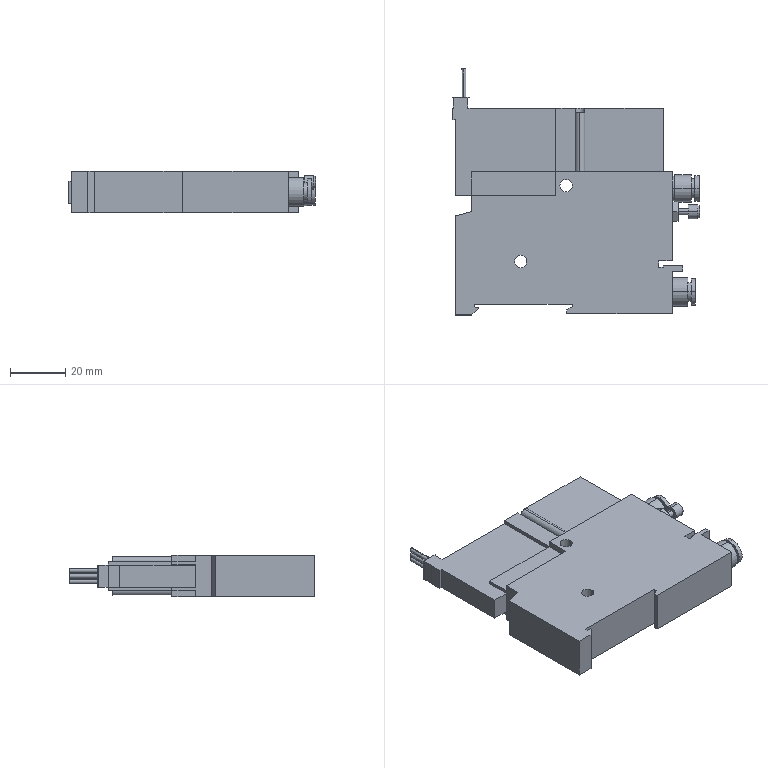Part | STEP file | 11-_ZK2A10KAL-06_BODY-V2.0011 | 1 solid | 134 faces | box 89.8 x 89.2 x 15.041 mm | volume 73976 mm3 | plane 93 | cylinder 40 | spline 1 | commonest cylinder face diameters 1.5 x6 3.5 x6 4.5 x4 6 x4 2.3 x2 4.4 x2